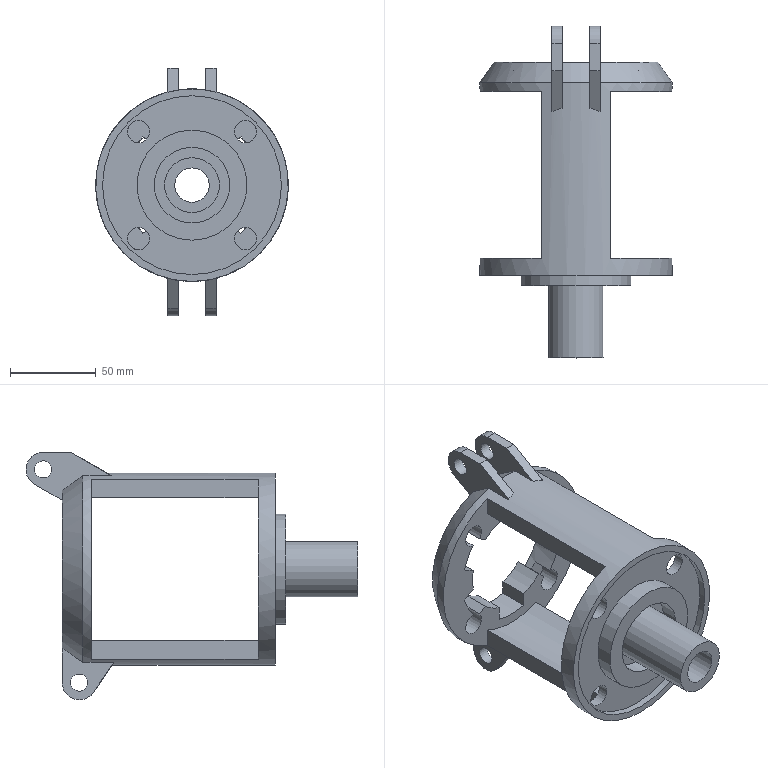Part | NX | features EXTRUDE 8, DATUM_CSYS 6, SKETCH 5, EXTRACT_STRING 4, CHAMFER 1, Instance Feature 1, Mirror Feature 1, REPLACE_FACE 1, SWP104 1, UNITE 1 | 1 solid | 84 faces | box 112 x 193 x 144 mm | volume 268281 mm3 | plane 44 | cylinder 36 | cone 4 | commonest cylinder face diameters 13 x8 64 x7 80 x6 20 x5 10 x4 92 x2